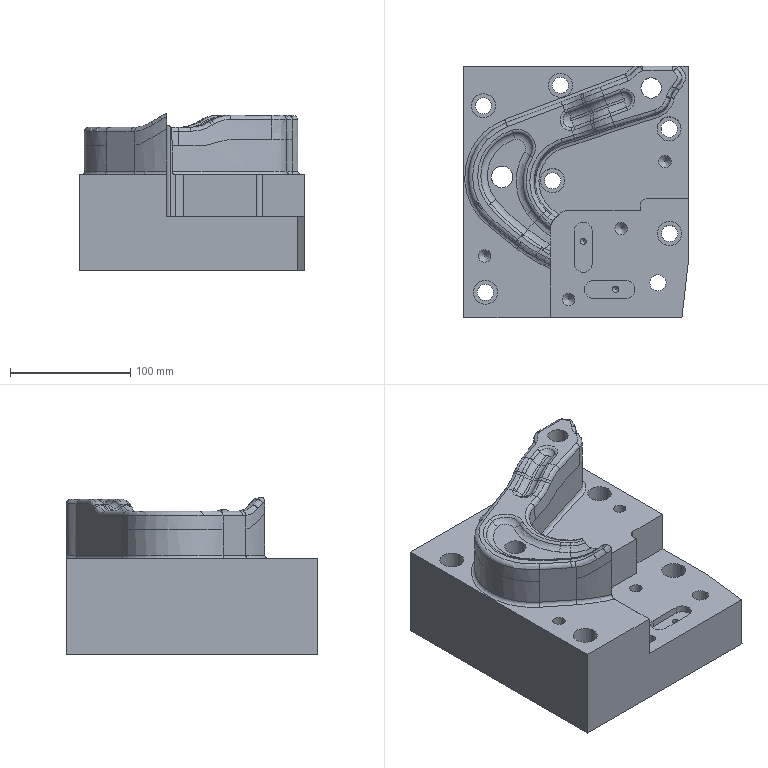Part | NX | features 23 2 | 1 solid | 183 faces | box 187 x 209 x 131.467 mm | volume 2940791 mm3 | cylinder 63 | spline 49 | plane 40 | torus 25 | cone 6 | commonest cylinder face diameters 20 x9 13.5 x7 6 x6 7 x6 10.3 x4 13 x4